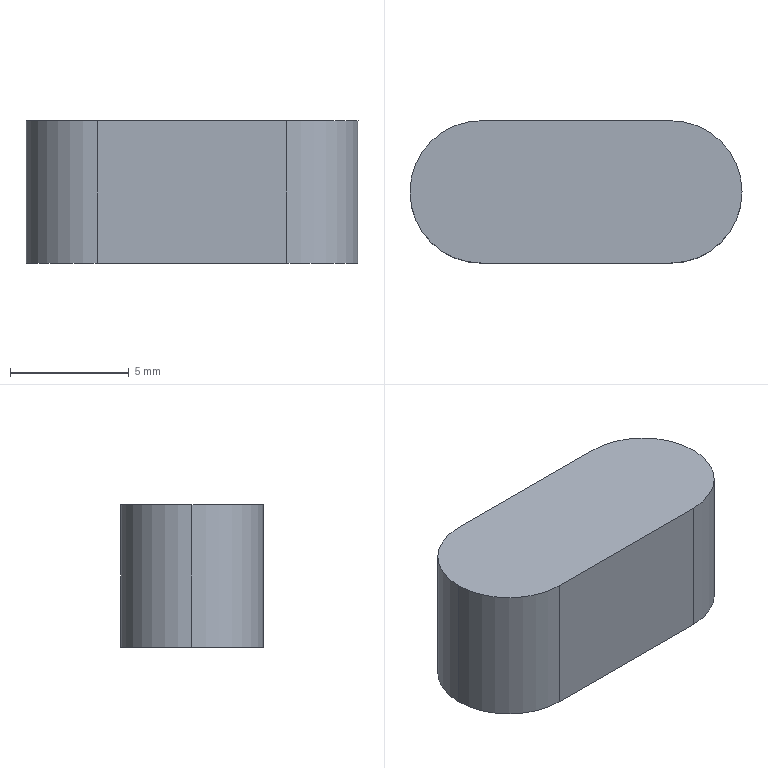Part | NX | features BREP 1 | 1 solid | 7 faces | box 14 x 6 x 6 mm | volume 457.646 mm3 | plane 4 | cylinder 3 | commonest cylinder face diameters 6 x3
STEP:
#1=CARTESIAN_POINT('',(-3.,0.,6.));
#2=VERTEX_POINT('',#1);
#3=CARTESIAN_POINT('',(0.,-3.,6.));
#4=VERTEX_POINT('',#3);
#5=CARTESIAN_POINT('',(0.,0.,6.));
#6=DIRECTION('',(0.,0.,1.));
#7=DIRECTION('',(1.,0.,0.));
#8=AXIS2_PLACEMENT_3D('',#5,#6,#7);
#9=CIRCLE('',#8,3.);
#10=EDGE_CURVE('',#2,#4,#9,.T.);
#11=ORIENTED_EDGE('',*,*,#10,.F.);
#12=CARTESIAN_POINT('',(-3.,0.,0.));
#13=VERTEX_POINT('',#12);
#14=CARTESIAN_POINT('',(-3.,0.,6.));
#15=DIRECTION('',(0.,0.,-1.));
#16=VECTOR('',#15,1000.);
#17=LINE('',#14,#16);
#18=EDGE_CURVE('',#2,#13,#17,.T.);
#19=ORIENTED_EDGE('',*,*,#18,.T.);
#20=CARTESIAN_POINT('',(0.,-3.,0.));
#21=VERTEX_POINT('',#20);
#22=CARTESIAN_POINT('',(0.,0.,0.));
#23=DIRECTION('',(0.,0.,1.));
#24=DIRECTION('',(1.,0.,0.));
#25=AXIS2_PLACEMENT_3D('',#22,#23,#24);
#26=CIRCLE('',#25,3.);
#27=EDGE_CURVE('',#13,#21,#26,.T.);
#28=ORIENTED_EDGE('',*,*,#27,.T.);
#29=CARTESIAN_POINT('',(0.,-3.,6.));
#30=DIRECTION('',(0.,0.,-1.));
#31=VECTOR('',#30,1000.);
#32=LINE('',#29,#31);
#33=EDGE_CURVE('',#4,#21,#32,.T.);
#34=ORIENTED_EDGE('',*,*,#33,.F.);
#35=EDGE_LOOP('',(#11,#19,#28,#34));
#36=FACE_BOUND('',#35,.T.);
#37=CARTESIAN_POINT('',(0.,0.,6.));
#38=DIRECTION('',(0.,0.,-1.));
#39=DIRECTION('',(1.,0.,0.));
#40=AXIS2_PLACEMENT_3D('',#37,#38,#39);
#41=CYLINDRICAL_SURFACE('',#40,3.);
#42=ADVANCED_FACE('',(#36),#41,.T.);
#43=ORIENTED_EDGE('',*,*,#18,.F.);
#44=CARTESIAN_POINT('',(0.,3.,6.));
#45=VERTEX_POINT('',#44);
#46=CARTESIAN_POINT('',(0.,0.,6.));
#47=DIRECTION('',(0.,0.,1.));
#48=DIRECTION('',(1.,0.,0.));
#49=AXIS2_PLACEMENT_3D('',#46,#47,#48);
#50=CIRCLE('',#49,3.);
#51=EDGE_CURVE('',#45,#2,#50,.T.);
#52=ORIENTED_EDGE('',*,*,#51,.F.);
#53=CARTESIAN_POINT('',(0.,3.,0.));
#54=VERTEX_POINT('',#53);
#55=CARTESIAN_POINT('',(0.,3.,6.));
#56=DIRECTION('',(0.,0.,-1.));
#57=VECTOR('',#56,1000.);
#58=LINE('',#55,#57);
#59=EDGE_CURVE('',#45,#54,#58,.T.);
#60=ORIENTED_EDGE('',*,*,#59,.T.);
#61=CARTESIAN_POINT('',(0.,0.,0.));
#62=DIRECTION('',(0.,0.,1.));
#63=DIRECTION('',(1.,0.,0.));
#64=AXIS2_PLACEMENT_3D('',#61,#62,#63);
#65=CIRCLE('',#64,3.);
#66=EDGE_CURVE('',#54,#13,#65,.T.);
#67=ORIENTED_EDGE('',*,*,#66,.T.);
#68=EDGE_LOOP('',(#43,#52,#60,#67));
#69=FACE_BOUND('',#68,.T.);
#70=CARTESIAN_POINT('',(0.,0.,6.));
#71=DIRECTION('',(0.,0.,-1.));
#72=DIRECTION('',(1.,0.,0.));
#73=AXIS2_PLACEMENT_3D('',#70,#71,#72);
#74=CYLINDRICAL_SURFACE('',#73,3.);
#75=ADVANCED_FACE('',(#69),#74,.T.);
#76=CARTESIAN_POINT('',(8.,-3.,0.));
#77=VERTEX_POINT('',#76);
#78=CARTESIAN_POINT('',(0.,-3.,0.));
#79=DIRECTION('',(1.,0.,0.));
#80=VECTOR('',#79,1000.);
#81=LINE('',#78,#80);
#82=EDGE_CURVE('',#21,#77,#81,.T.);
#83=ORIENTED_EDGE('',*,*,#82,.T.);
#84=CARTESIAN_POINT('',(8.,-3.,6.));
#85=VERTEX_POINT('',#84);
#86=CARTESIAN_POINT('',(8.,-3.,6.));
#87=DIRECTION('',(0.,0.,-1.));
#88=VECTOR('',#87,1000.);
#89=LINE('',#86,#88);
#90=EDGE_CURVE('',#85,#77,#89,.T.);
#91=ORIENTED_EDGE('',*,*,#90,.F.);
#92=CARTESIAN_POINT('',(0.,-3.,6.));
#93=DIRECTION('',(1.,0.,0.));
#94=VECTOR('',#93,1000.);
#95=LINE('',#92,#94);
#96=EDGE_CURVE('',#4,#85,#95,.T.);
#97=ORIENTED_EDGE('',*,*,#96,.F.);
#98=ORIENTED_EDGE('',*,*,#33,.T.);
#99=EDGE_LOOP('',(#83,#91,#97,#98));
#100=FACE_BOUND('',#99,.T.);
#101=CARTESIAN_POINT('',(0.,-3.,6.));
#102=DIRECTION('',(0.,1.,0.));
#103=DIRECTION('',(0.,0.,1.));
#104=AXIS2_PLACEMENT_3D('',#101,#102,#103);
#105=PLANE('',#104);
#106=ADVANCED_FACE('',(#100),#105,.F.);
#107=CARTESIAN_POINT('',(8.,3.,0.));
#108=VERTEX_POINT('',#107);
#109=CARTESIAN_POINT('',(8.,0.,0.));
#110=DIRECTION('',(0.,0.,1.));
#111=DIRECTION('',(1.,0.,0.));
#112=AXIS2_PLACEMENT_3D('',#109,#110,#111);
#113=CIRCLE('',#112,3.);
#114=EDGE_CURVE('',#77,#108,#113,.T.);
#115=ORIENTED_EDGE('',*,*,#114,.T.);
#116=CARTESIAN_POINT('',(8.,3.,6.));
#117=VERTEX_POINT('',#116);
#118=CARTESIAN_POINT('',(8.,3.,6.));
#119=DIRECTION('',(0.,0.,-1.));
#120=VECTOR('',#119,1000.);
#121=LINE('',#118,#120);
#122=EDGE_CURVE('',#117,#108,#121,.T.);
#123=ORIENTED_EDGE('',*,*,#122,.F.);
#124=CARTESIAN_POINT('',(8.,0.,6.));
#125=DIRECTION('',(0.,0.,1.));
#126=DIRECTION('',(1.,0.,0.));
#127=AXIS2_PLACEMENT_3D('',#124,#125,#126);
#128=CIRCLE('',#127,3.);
#129=EDGE_CURVE('',#85,#117,#128,.T.);
#130=ORIENTED_EDGE('',*,*,#129,.F.);
#131=ORIENTED_EDGE('',*,*,#90,.T.);
#132=EDGE_LOOP('',(#115,#123,#130,#131));
#133=FACE_BOUND('',#132,.T.);
#134=CARTESIAN_POINT('',(8.,0.,6.));
#135=DIRECTION('',(0.,0.,-1.));
#136=DIRECTION('',(1.,0.,0.));
#137=AXIS2_PLACEMENT_3D('',#134,#135,#136);
#138=CYLINDRICAL_SURFACE('',#137,3.);
#139=ADVANCED_FACE('',(#133),#138,.T.);
#140=CARTESIAN_POINT('',(0.,3.,0.));
#141=DIRECTION('',(-1.,0.,0.));
#142=VECTOR('',#141,1000.);
#143=LINE('',#140,#142);
#144=EDGE_CURVE('',#108,#54,#143,.T.);
#145=ORIENTED_EDGE('',*,*,#144,.T.);
#146=ORIENTED_EDGE('',*,*,#59,.F.);
#147=CARTESIAN_POINT('',(0.,3.,6.));
#148=DIRECTION('',(-1.,0.,0.));
#149=VECTOR('',#148,1000.);
#150=LINE('',#147,#149);
#151=EDGE_CURVE('',#117,#45,#150,.T.);
#152=ORIENTED_EDGE('',*,*,#151,.F.);
#153=ORIENTED_EDGE('',*,*,#122,.T.);
#154=EDGE_LOOP('',(#145,#146,#152,#153));
#155=FACE_BOUND('',#154,.T.);
#156=CARTESIAN_POINT('',(0.,3.,6.));
#157=DIRECTION('',(0.,-1.,0.));
#158=DIRECTION('',(0.,0.,1.));
#159=AXIS2_PLACEMENT_3D('',#156,#157,#158);
#160=PLANE('',#159);
#161=ADVANCED_FACE('',(#155),#160,.F.);
#162=ORIENTED_EDGE('',*,*,#51,.T.);
#163=ORIENTED_EDGE('',*,*,#10,.T.);
#164=ORIENTED_EDGE('',*,*,#96,.T.);
#165=ORIENTED_EDGE('',*,*,#129,.T.);
#166=ORIENTED_EDGE('',*,*,#151,.T.);
#167=EDGE_LOOP('',(#162,#163,#164,#165,#166));
#168=FACE_BOUND('',#167,.T.);
#169=CARTESIAN_POINT('',(0.,0.,6.));
#170=DIRECTION('',(0.,0.,1.));
#171=DIRECTION('',(0.,1.,0.));
#172=AXIS2_PLACEMENT_3D('',#169,#170,#171);
#173=PLANE('',#172);
#174=ADVANCED_FACE('',(#168),#173,.T.);
#175=ORIENTED_EDGE('',*,*,#66,.F.);
#176=ORIENTED_EDGE('',*,*,#144,.F.);
#177=ORIENTED_EDGE('',*,*,#114,.F.);
#178=ORIENTED_EDGE('',*,*,#82,.F.);
#179=ORIENTED_EDGE('',*,*,#27,.F.);
#180=EDGE_LOOP('',(#175,#176,#177,#178,#179));
#181=FACE_BOUND('',#180,.T.);
#182=CARTESIAN_POINT('',(0.,0.,0.));
#183=DIRECTION('',(0.,0.,1.));
#184=DIRECTION('',(0.,1.,0.));
#185=AXIS2_PLACEMENT_3D('',#182,#183,#184);
#186=PLANE('',#185);
#187=ADVANCED_FACE('',(#181),#186,.F.);
#188=CLOSED_SHELL('',(#42,#75,#106,#139,#161,#174,#187));
#189=MANIFOLD_SOLID_BREP('',#188);
#190=(LENGTH_UNIT()NAMED_UNIT(*)SI_UNIT(.MILLI.,.METRE.));
#191=UNCERTAINTY_MEASURE_WITH_UNIT(LENGTH_MEASURE(0.00001),#190,'','');
#192=(NAMED_UNIT(*)PLANE_ANGLE_UNIT()SI_UNIT($,.RADIAN.));
#193=(NAMED_UNIT(*)SI_UNIT($,.STERADIAN.)SOLID_ANGLE_UNIT());
#194=(GEOMETRIC_REPRESENTATION_CONTEXT(3)GLOBAL_UNCERTAINTY_ASSIGNED_CONTEXT((#191))GLOBAL_UNIT_ASSIGNED_CONTEXT((#190,#192,#193))REPRESENTATION_CONTEXT('',''));
#195=ADVANCED_BREP_SHAPE_REPRESENTATION('',(#189),#194);